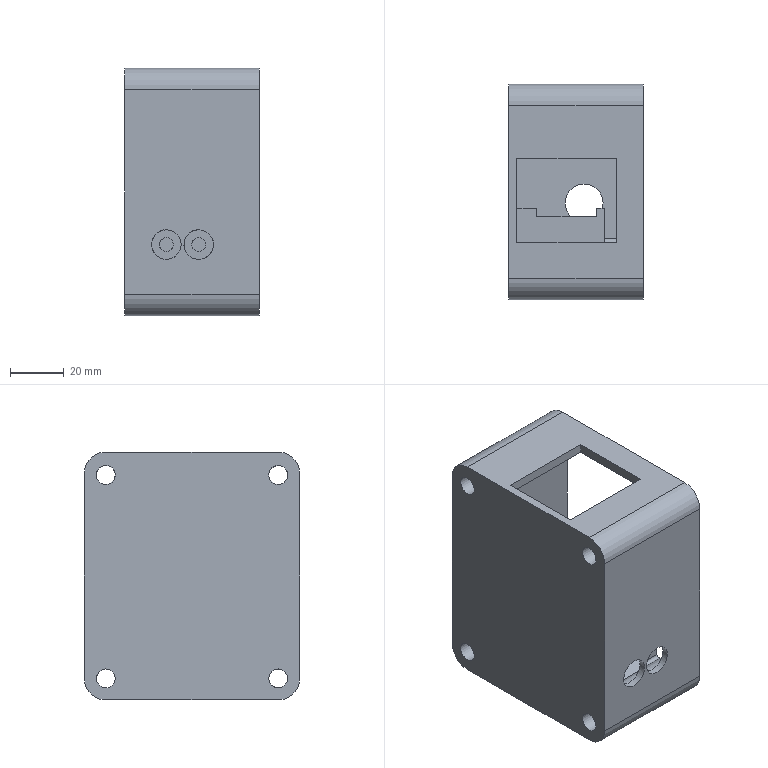NC program | NX | posted by the shop | part box 50 x 80 x 92 mm
Whole program:
%
O1234(2)
(T=1 D63 face mill Z=-30.00 D=63.00 R=0.00 L=30.00)
()
G40 G17 G80 G90 G21
M9
M5
G91 G28 Z0.0
M1
N1
(T=1 N=D63 face mill D=1.00 R=0.00 FL=10.00 L=11.00)
(XY-STOCK=0.05)
T1 M6
T12
G0 G90 G54 X101. Y-19.3 S3500 M3
G43 H01 Z20.
M8
Z11.258
G1 Z8.258 F1000.
X38.
X-38.
X-101.
Z11.258
G0 Z20.
X101. Y18.5
Z11.258
G1 Z8.258
X38.
X-38.
X-101.
Z11.258
G0 Z20.
X101. Y-19.3
Z10.517
G1 Z7.517
X38.
X-38.
X-101.
Z10.517
G0 Z20.
X101. Y18.5
Z10.517
G1 Z7.517
X38.
X-38.
X-101.
Z10.517
G0 Z20.
X101. Y-19.3
Z9.775
G1 Z6.775
X38.
X-38.
X-101.
Z9.775
G0 Z20.
X101. Y18.5
Z9.775
G1 Z6.775
X38.
X-38.
X-101.
Z9.775
G0 Z20.
X101. Y-19.3
Z9.033
G1 Z6.033
X38.
X-38.
X-101.
Z9.033
G0 Z20.
X101. Y18.5
Z9.033
G1 Z6.033
X38.
X-38.
X-101.
Z9.033
G0 Z20.
X101. Y-19.3
Z8.292
G1 Z5.292
X38.
X-38.
X-101.
Z8.292
G0 Z20.
X101. Y18.5
Z8.292
G1 Z5.292
X38.
X-38.
X-101.
Z8.292
G0 Z20.
X101. Y-19.3
Z7.55
G1 Z4.55
X38.
X-38.
X-101.
Z7.55
G0 Z20.
X101. Y18.5
Z7.55
G1 Z4.55
X38.
X-38.
X-101.
Z7.55
G0 Z20.
X101. Y-19.3
Z6.808
G1 Z3.808
X38.
X-38.
X-101.
Z6.808
G0 Z20.
X101. Y18.5
Z6.808
G1 Z3.808
X38.
X-38.
X-101.
Z6.808
G0 Z20.
X101. Y-19.3
Z6.067
G1 Z3.067
X38.
X-38.
X-101.
Z6.067
G0 Z20.
X101. Y18.5
Z6.067
G1 Z3.067
X38.
X-38.
X-101.
Z6.067
G0 Z20.
X101. Y-19.3
Z5.325
G1 Z2.325
X38.
X-38.
X-101.
Z5.325
G0 Z20.
X101. Y18.5
Z5.325
G1 Z2.325
X38.
X-38.
X-101.
Z5.325
G0 Z20.
X101. Y-19.3
Z4.583
G1 Z1.583
X38.
X-38.
X-101.
Z4.583
G0 Z20.
X101. Y18.5
Z4.583
G1 Z1.583
X38.
X-38.
X-101.
Z4.583
G0 Z20.
X101. Y-19.3
Z3.842
G1 Z.842
X38.
X-38.
X-101.
Z3.842
G0 Z20.
X101. Y18.5
Z3.842
G1 Z.842
X38.
X-38.
X-101.
Z3.842
G0 Z20.
X101. Y-19.3
Z3.1
G1 Z.1
X38.
X-38.
X-101.
Z3.1
G0 Z20.
X101. Y18.5
Z3.1
G1 Z.1
X38.
X-38.
X-101.
Z3.1
G0 Z20.
G0 X101. Y-19.3 S3500 M3
M8
Z3.
G1 Z0.0 F600.
X38.
X-38.
X-101.
Z3.
G0 Z20.
X101. Y18.5
Z3.
G1 Z0.0
X38.
X-38.
X-101.
Z3.
G0 Z20.
M9
M5
G91 G28 Z0.0
M1
N2
(T=12 N=倒角D5-90度 D=5.00 R=0.00 FL=5.00 L=50.00)
(XY-STOCK=0.00)
T12 M6
T1
G0 G90 G54 X-2. Y44. S3500 M3
G43 H12 Z20.
M8
Z0.0
G1 Z-2. F1000.
G3 X0.0 Y42. I2. J0.0
G1 X38.
G2 X48. Y32. I0.0 J-10.
G1 Y-32.
G2 X38. Y-42. I-10. J0.0
G1 X-38.
G2 X-48. Y-32. I0.0 J10.
G1 Y32.
G2 X-38. Y42. I10. J0.0
G1 X0.0
G3 X2. Y44. I0.0 J2.
G1 Z0.0
G0 Z20.
G0 X38. Y-31. S3500 M3
M8
Z.5
G1 Z-1.5 F800.
X37.
G3 X36. Y-32. I0.0 J-1.
I2. J0.0
X37. Y-33. I1. J0.0
G1 X38.
Z.5
G0 Z20.
Y33.
Z.5
G1 Z-1.5
X37.
G3 X36. Y32. I0.0 J-1.
I2. J0.0
X37. Y31. I1. J0.0
G1 X38.
Z.5
G0 Z20.
X-37.5 Y33.
Z.5
G1 Z-1.5
X-38.5
G3 X-39.5 Y32. I0.0 J-1.
I2. J0.0
X-38.5 Y31. I1. J0.0
G1 X-37.5
Z.5
G0 Z20.
Y-31.
Z.5
G1 Z-1.5
X-38.5
G3 X-39.5 Y-32. I0.0 J-1.
I2. J0.0
X-38.5 Y-33. I1. J0.0
G1 X-37.5
Z.5
G0 Z20.
M9
M5
G91 G28 Z0.0
G28 Y0.
M30
%